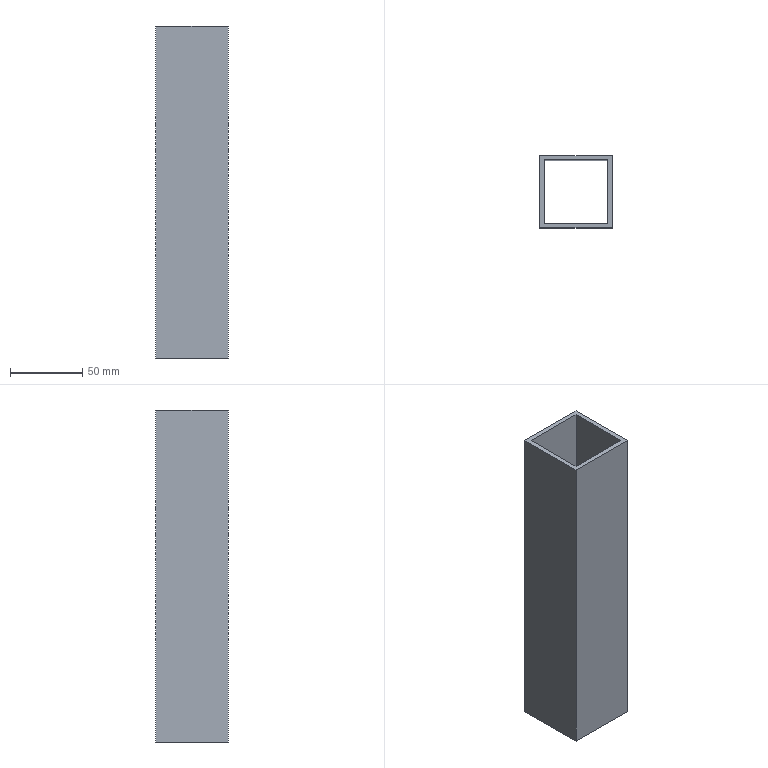Part | STEP file | BCC3 H19_1 | 1 solid | 10 faces | box 50 x 50 x 230 mm | volume 129720 mm3 | plane 10
STEP:
#1=CARTESIAN_POINT('',(0.,0.,0.));
#2=DIRECTION('',(0.,0.,1.));
#3=DIRECTION('',(1.,0.,0.));
#4=AXIS2_PLACEMENT_3D('',#1,#2,#3);
#5=CARTESIAN_POINT('',(-25.,25.,115.));
#6=VERTEX_POINT('',#5);
#7=CARTESIAN_POINT('',(-25.,-25.,115.));
#8=VERTEX_POINT('',#7);
#9=CARTESIAN_POINT('',(-25.,25.,115.));
#10=DIRECTION('',(0.,-1.,0.));
#11=VECTOR('',#10,1.);
#12=LINE('',#9,#11);
#13=CARTESIAN_POINT('',(0.,0.,115.));
#14=DIRECTION('',(0.,0.,1.));
#15=DIRECTION('',(1.,0.,0.));
#16=AXIS2_PLACEMENT_3D('',#13,#14,#15);
#17=PLANE('',#16);
#18=CARTESIAN_POINT('',(-25.,25.));
#19=DIRECTION('',(0.,-1.));
#20=VECTOR('',#19,1.);
#21=LINE('',#18,#20);
#22=(GEOMETRIC_REPRESENTATION_CONTEXT(2)PARAMETRIC_REPRESENTATION_CONTEXT()REPRESENTATION_CONTEXT('',''));
#23=DEFINITIONAL_REPRESENTATION('',(#21),#22);
#24=PCURVE('',#17,#23);
#25=CARTESIAN_POINT('',(-25.,25.,115.));
#26=DIRECTION('',(1.,0.,0.));
#27=DIRECTION('',(0.,1.,0.));
#28=AXIS2_PLACEMENT_3D('',#25,#26,#27);
#29=PLANE('',#28);
#30=CARTESIAN_POINT('',(0.,0.));
#31=DIRECTION('',(-1.,0.));
#32=VECTOR('',#31,1.);
#33=LINE('',#30,#32);
#34=(GEOMETRIC_REPRESENTATION_CONTEXT(2)PARAMETRIC_REPRESENTATION_CONTEXT()REPRESENTATION_CONTEXT('',''));
#35=DEFINITIONAL_REPRESENTATION('',(#33),#34);
#36=PCURVE('',#29,#35);
#37=SURFACE_CURVE('',#12,(#24,#36),.PCURVE_S1.);
#38=EDGE_CURVE('',#6,#8,#37,.T.);
#39=ORIENTED_EDGE('',*,*,#38,.T.);
#40=CARTESIAN_POINT('',(25.,-25.,115.));
#41=VERTEX_POINT('',#40);
#42=CARTESIAN_POINT('',(-25.,-25.,115.));
#43=DIRECTION('',(1.,0.,0.));
#44=VECTOR('',#43,1.);
#45=LINE('',#42,#44);
#46=CARTESIAN_POINT('',(-25.,-25.));
#47=DIRECTION('',(1.,0.));
#48=VECTOR('',#47,1.);
#49=LINE('',#46,#48);
#50=(GEOMETRIC_REPRESENTATION_CONTEXT(2)PARAMETRIC_REPRESENTATION_CONTEXT()REPRESENTATION_CONTEXT('',''));
#51=DEFINITIONAL_REPRESENTATION('',(#49),#50);
#52=PCURVE('',#17,#51);
#53=CARTESIAN_POINT('',(-25.,-25.,115.));
#54=DIRECTION('',(0.,1.,0.));
#55=DIRECTION('',(0.,0.,1.));
#56=AXIS2_PLACEMENT_3D('',#53,#54,#55);
#57=PLANE('',#56);
#58=CARTESIAN_POINT('',(0.,0.));
#59=DIRECTION('',(0.,1.));
#60=VECTOR('',#59,1.);
#61=LINE('',#58,#60);
#62=(GEOMETRIC_REPRESENTATION_CONTEXT(2)PARAMETRIC_REPRESENTATION_CONTEXT()REPRESENTATION_CONTEXT('',''));
#63=DEFINITIONAL_REPRESENTATION('',(#61),#62);
#64=PCURVE('',#57,#63);
#65=SURFACE_CURVE('',#45,(#52,#64),.PCURVE_S1.);
#66=EDGE_CURVE('',#8,#41,#65,.T.);
#67=ORIENTED_EDGE('',*,*,#66,.T.);
#68=CARTESIAN_POINT('',(25.,25.,115.));
#69=VERTEX_POINT('',#68);
#70=CARTESIAN_POINT('',(25.,25.,115.));
#71=DIRECTION('',(0.,1.,0.));
#72=VECTOR('',#71,1.);
#73=LINE('',#70,#72);
#74=CARTESIAN_POINT('',(25.,25.));
#75=DIRECTION('',(0.,1.));
#76=VECTOR('',#75,1.);
#77=LINE('',#74,#76);
#78=(GEOMETRIC_REPRESENTATION_CONTEXT(2)PARAMETRIC_REPRESENTATION_CONTEXT()REPRESENTATION_CONTEXT('',''));
#79=DEFINITIONAL_REPRESENTATION('',(#77),#78);
#80=PCURVE('',#17,#79);
#81=CARTESIAN_POINT('',(25.,25.,115.));
#82=DIRECTION('',(-1.,0.,0.));
#83=DIRECTION('',(0.,-1.,0.));
#84=AXIS2_PLACEMENT_3D('',#81,#82,#83);
#85=PLANE('',#84);
#86=CARTESIAN_POINT('',(0.,0.));
#87=DIRECTION('',(-1.,0.));
#88=VECTOR('',#87,1.);
#89=LINE('',#86,#88);
#90=(GEOMETRIC_REPRESENTATION_CONTEXT(2)PARAMETRIC_REPRESENTATION_CONTEXT()REPRESENTATION_CONTEXT('',''));
#91=DEFINITIONAL_REPRESENTATION('',(#89),#90);
#92=PCURVE('',#85,#91);
#93=SURFACE_CURVE('',#73,(#80,#92),.PCURVE_S1.);
#94=EDGE_CURVE('',#41,#69,#93,.T.);
#95=ORIENTED_EDGE('',*,*,#94,.T.);
#96=CARTESIAN_POINT('',(-25.,25.,115.));
#97=DIRECTION('',(-1.,0.,0.));
#98=VECTOR('',#97,1.);
#99=LINE('',#96,#98);
#100=CARTESIAN_POINT('',(-25.,25.));
#101=DIRECTION('',(-1.,0.));
#102=VECTOR('',#101,1.);
#103=LINE('',#100,#102);
#104=(GEOMETRIC_REPRESENTATION_CONTEXT(2)PARAMETRIC_REPRESENTATION_CONTEXT()REPRESENTATION_CONTEXT('',''));
#105=DEFINITIONAL_REPRESENTATION('',(#103),#104);
#106=PCURVE('',#17,#105);
#107=CARTESIAN_POINT('',(-25.,25.,115.));
#108=DIRECTION('',(0.,-1.,0.));
#109=DIRECTION('',(0.,0.,-1.));
#110=AXIS2_PLACEMENT_3D('',#107,#108,#109);
#111=PLANE('',#110);
#112=CARTESIAN_POINT('',(0.,0.));
#113=DIRECTION('',(0.,-1.));
#114=VECTOR('',#113,1.);
#115=LINE('',#112,#114);
#116=(GEOMETRIC_REPRESENTATION_CONTEXT(2)PARAMETRIC_REPRESENTATION_CONTEXT()REPRESENTATION_CONTEXT('',''));
#117=DEFINITIONAL_REPRESENTATION('',(#115),#116);
#118=PCURVE('',#111,#117);
#119=SURFACE_CURVE('',#99,(#106,#118),.PCURVE_S1.);
#120=EDGE_CURVE('',#69,#6,#119,.T.);
#121=ORIENTED_EDGE('',*,*,#120,.T.);
#122=EDGE_LOOP('',(#39,#67,#95,#121));
#123=FACE_BOUND('',#122,.T.);
#124=CARTESIAN_POINT('',(-22.,-22.,115.));
#125=VERTEX_POINT('',#124);
#126=CARTESIAN_POINT('',(22.,-22.,115.));
#127=VERTEX_POINT('',#126);
#128=CARTESIAN_POINT('',(-22.,-22.,115.));
#129=DIRECTION('',(1.,0.,0.));
#130=VECTOR('',#129,1.);
#131=LINE('',#128,#130);
#132=CARTESIAN_POINT('',(-22.,-22.));
#133=DIRECTION('',(1.,0.));
#134=VECTOR('',#133,1.);
#135=LINE('',#132,#134);
#136=(GEOMETRIC_REPRESENTATION_CONTEXT(2)PARAMETRIC_REPRESENTATION_CONTEXT()REPRESENTATION_CONTEXT('',''));
#137=DEFINITIONAL_REPRESENTATION('',(#135),#136);
#138=PCURVE('',#17,#137);
#139=CARTESIAN_POINT('',(-22.,-22.,115.));
#140=DIRECTION('',(0.,1.,0.));
#141=DIRECTION('',(-1.,0.,0.));
#142=AXIS2_PLACEMENT_3D('',#139,#140,#141);
#143=PLANE('',#142);
#144=CARTESIAN_POINT('',(0.,0.));
#145=DIRECTION('',(-1.,0.));
#146=VECTOR('',#145,1.);
#147=LINE('',#144,#146);
#148=(GEOMETRIC_REPRESENTATION_CONTEXT(2)PARAMETRIC_REPRESENTATION_CONTEXT()REPRESENTATION_CONTEXT('',''));
#149=DEFINITIONAL_REPRESENTATION('',(#147),#148);
#150=PCURVE('',#143,#149);
#151=SURFACE_CURVE('',#131,(#138,#150),.PCURVE_S1.);
#152=EDGE_CURVE('',#125,#127,#151,.T.);
#153=ORIENTED_EDGE('',*,*,#152,.F.);
#154=CARTESIAN_POINT('',(-22.,22.,115.));
#155=VERTEX_POINT('',#154);
#156=CARTESIAN_POINT('',(-22.,22.,115.));
#157=DIRECTION('',(0.,-1.,0.));
#158=VECTOR('',#157,1.);
#159=LINE('',#156,#158);
#160=CARTESIAN_POINT('',(-22.,22.));
#161=DIRECTION('',(0.,-1.));
#162=VECTOR('',#161,1.);
#163=LINE('',#160,#162);
#164=(GEOMETRIC_REPRESENTATION_CONTEXT(2)PARAMETRIC_REPRESENTATION_CONTEXT()REPRESENTATION_CONTEXT('',''));
#165=DEFINITIONAL_REPRESENTATION('',(#163),#164);
#166=PCURVE('',#17,#165);
#167=CARTESIAN_POINT('',(-22.,22.,115.));
#168=DIRECTION('',(1.,0.,0.));
#169=DIRECTION('',(0.,1.,0.));
#170=AXIS2_PLACEMENT_3D('',#167,#168,#169);
#171=PLANE('',#170);
#172=CARTESIAN_POINT('',(0.,0.));
#173=DIRECTION('',(-1.,0.));
#174=VECTOR('',#173,1.);
#175=LINE('',#172,#174);
#176=(GEOMETRIC_REPRESENTATION_CONTEXT(2)PARAMETRIC_REPRESENTATION_CONTEXT()REPRESENTATION_CONTEXT('',''));
#177=DEFINITIONAL_REPRESENTATION('',(#175),#176);
#178=PCURVE('',#171,#177);
#179=SURFACE_CURVE('',#159,(#166,#178),.PCURVE_S1.);
#180=EDGE_CURVE('',#155,#125,#179,.T.);
#181=ORIENTED_EDGE('',*,*,#180,.F.);
#182=CARTESIAN_POINT('',(22.,22.,115.));
#183=VERTEX_POINT('',#182);
#184=CARTESIAN_POINT('',(-22.,22.,115.));
#185=DIRECTION('',(-1.,0.,0.));
#186=VECTOR('',#185,1.);
#187=LINE('',#184,#186);
#188=CARTESIAN_POINT('',(-22.,22.));
#189=DIRECTION('',(-1.,0.));
#190=VECTOR('',#189,1.);
#191=LINE('',#188,#190);
#192=(GEOMETRIC_REPRESENTATION_CONTEXT(2)PARAMETRIC_REPRESENTATION_CONTEXT()REPRESENTATION_CONTEXT('',''));
#193=DEFINITIONAL_REPRESENTATION('',(#191),#192);
#194=PCURVE('',#17,#193);
#195=CARTESIAN_POINT('',(-22.,22.,115.));
#196=DIRECTION('',(0.,-1.,0.));
#197=DIRECTION('',(0.,0.,-1.));
#198=AXIS2_PLACEMENT_3D('',#195,#196,#197);
#199=PLANE('',#198);
#200=CARTESIAN_POINT('',(0.,0.));
#201=DIRECTION('',(0.,-1.));
#202=VECTOR('',#201,1.);
#203=LINE('',#200,#202);
#204=(GEOMETRIC_REPRESENTATION_CONTEXT(2)PARAMETRIC_REPRESENTATION_CONTEXT()REPRESENTATION_CONTEXT('',''));
#205=DEFINITIONAL_REPRESENTATION('',(#203),#204);
#206=PCURVE('',#199,#205);
#207=SURFACE_CURVE('',#187,(#194,#206),.PCURVE_S1.);
#208=EDGE_CURVE('',#183,#155,#207,.T.);
#209=ORIENTED_EDGE('',*,*,#208,.F.);
#210=CARTESIAN_POINT('',(22.,22.,115.));
#211=DIRECTION('',(0.,1.,0.));
#212=VECTOR('',#211,1.);
#213=LINE('',#210,#212);
#214=CARTESIAN_POINT('',(22.,22.));
#215=DIRECTION('',(0.,1.));
#216=VECTOR('',#215,1.);
#217=LINE('',#214,#216);
#218=(GEOMETRIC_REPRESENTATION_CONTEXT(2)PARAMETRIC_REPRESENTATION_CONTEXT()REPRESENTATION_CONTEXT('',''));
#219=DEFINITIONAL_REPRESENTATION('',(#217),#218);
#220=PCURVE('',#17,#219);
#221=CARTESIAN_POINT('',(22.,22.,115.));
#222=DIRECTION('',(-1.,0.,0.));
#223=DIRECTION('',(0.,-1.,0.));
#224=AXIS2_PLACEMENT_3D('',#221,#222,#223);
#225=PLANE('',#224);
#226=CARTESIAN_POINT('',(0.,0.));
#227=DIRECTION('',(-1.,0.));
#228=VECTOR('',#227,1.);
#229=LINE('',#226,#228);
#230=(GEOMETRIC_REPRESENTATION_CONTEXT(2)PARAMETRIC_REPRESENTATION_CONTEXT()REPRESENTATION_CONTEXT('',''));
#231=DEFINITIONAL_REPRESENTATION('',(#229),#230);
#232=PCURVE('',#225,#231);
#233=SURFACE_CURVE('',#213,(#220,#232),.PCURVE_S1.);
#234=EDGE_CURVE('',#127,#183,#233,.T.);
#235=ORIENTED_EDGE('',*,*,#234,.F.);
#236=EDGE_LOOP('',(#153,#181,#209,#235));
#237=FACE_BOUND('',#236,.T.);
#238=ADVANCED_FACE('',(#123,#237),#17,.T.);
#239=CARTESIAN_POINT('',(-25.,25.,-115.));
#240=VERTEX_POINT('',#239);
#241=CARTESIAN_POINT('',(-25.,-25.,-115.));
#242=VERTEX_POINT('',#241);
#243=CARTESIAN_POINT('',(-25.,25.,-115.));
#244=DIRECTION('',(0.,-1.,0.));
#245=VECTOR('',#244,1.);
#246=LINE('',#243,#245);
#247=CARTESIAN_POINT('',(0.,0.,-115.));
#248=DIRECTION('',(0.,0.,1.));
#249=DIRECTION('',(1.,0.,0.));
#250=AXIS2_PLACEMENT_3D('',#247,#248,#249);
#251=PLANE('',#250);
#252=CARTESIAN_POINT('',(-25.,25.));
#253=DIRECTION('',(0.,-1.));
#254=VECTOR('',#253,1.);
#255=LINE('',#252,#254);
#256=(GEOMETRIC_REPRESENTATION_CONTEXT(2)PARAMETRIC_REPRESENTATION_CONTEXT()REPRESENTATION_CONTEXT('',''));
#257=DEFINITIONAL_REPRESENTATION('',(#255),#256);
#258=PCURVE('',#251,#257);
#259=CARTESIAN_POINT('',(0.,-230.));
#260=DIRECTION('',(-1.,0.));
#261=VECTOR('',#260,1.);
#262=LINE('',#259,#261);
#263=(GEOMETRIC_REPRESENTATION_CONTEXT(2)PARAMETRIC_REPRESENTATION_CONTEXT()REPRESENTATION_CONTEXT('',''));
#264=DEFINITIONAL_REPRESENTATION('',(#262),#263);
#265=PCURVE('',#29,#264);
#266=SURFACE_CURVE('',#246,(#258,#265),.PCURVE_S1.);
#267=EDGE_CURVE('',#240,#242,#266,.T.);
#268=ORIENTED_EDGE('',*,*,#267,.F.);
#269=CARTESIAN_POINT('',(25.,25.,-115.));
#270=VERTEX_POINT('',#269);
#271=CARTESIAN_POINT('',(-25.,25.,-115.));
#272=DIRECTION('',(-1.,0.,0.));
#273=VECTOR('',#272,1.);
#274=LINE('',#271,#273);
#275=CARTESIAN_POINT('',(-25.,25.));
#276=DIRECTION('',(-1.,0.));
#277=VECTOR('',#276,1.);
#278=LINE('',#275,#277);
#279=(GEOMETRIC_REPRESENTATION_CONTEXT(2)PARAMETRIC_REPRESENTATION_CONTEXT()REPRESENTATION_CONTEXT('',''));
#280=DEFINITIONAL_REPRESENTATION('',(#278),#279);
#281=PCURVE('',#251,#280);
#282=CARTESIAN_POINT('',(230.,0.));
#283=DIRECTION('',(0.,-1.));
#284=VECTOR('',#283,1.);
#285=LINE('',#282,#284);
#286=(GEOMETRIC_REPRESENTATION_CONTEXT(2)PARAMETRIC_REPRESENTATION_CONTEXT()REPRESENTATION_CONTEXT('',''));
#287=DEFINITIONAL_REPRESENTATION('',(#285),#286);
#288=PCURVE('',#111,#287);
#289=SURFACE_CURVE('',#274,(#281,#288),.PCURVE_S1.);
#290=EDGE_CURVE('',#270,#240,#289,.T.);
#291=ORIENTED_EDGE('',*,*,#290,.F.);
#292=CARTESIAN_POINT('',(25.,-25.,-115.));
#293=VERTEX_POINT('',#292);
#294=CARTESIAN_POINT('',(25.,25.,-115.));
#295=DIRECTION('',(0.,1.,0.));
#296=VECTOR('',#295,1.);
#297=LINE('',#294,#296);
#298=CARTESIAN_POINT('',(25.,25.));
#299=DIRECTION('',(0.,1.));
#300=VECTOR('',#299,1.);
#301=LINE('',#298,#300);
#302=(GEOMETRIC_REPRESENTATION_CONTEXT(2)PARAMETRIC_REPRESENTATION_CONTEXT()REPRESENTATION_CONTEXT('',''));
#303=DEFINITIONAL_REPRESENTATION('',(#301),#302);
#304=PCURVE('',#251,#303);
#305=CARTESIAN_POINT('',(0.,-230.));
#306=DIRECTION('',(-1.,0.));
#307=VECTOR('',#306,1.);
#308=LINE('',#305,#307);
#309=(GEOMETRIC_REPRESENTATION_CONTEXT(2)PARAMETRIC_REPRESENTATION_CONTEXT()REPRESENTATION_CONTEXT('',''));
#310=DEFINITIONAL_REPRESENTATION('',(#308),#309);
#311=PCURVE('',#85,#310);
#312=SURFACE_CURVE('',#297,(#304,#311),.PCURVE_S1.);
#313=EDGE_CURVE('',#293,#270,#312,.T.);
#314=ORIENTED_EDGE('',*,*,#313,.F.);
#315=CARTESIAN_POINT('',(-25.,-25.,-115.));
#316=DIRECTION('',(1.,0.,0.));
#317=VECTOR('',#316,1.);
#318=LINE('',#315,#317);
#319=CARTESIAN_POINT('',(-25.,-25.));
#320=DIRECTION('',(1.,0.));
#321=VECTOR('',#320,1.);
#322=LINE('',#319,#321);
#323=(GEOMETRIC_REPRESENTATION_CONTEXT(2)PARAMETRIC_REPRESENTATION_CONTEXT()REPRESENTATION_CONTEXT('',''));
#324=DEFINITIONAL_REPRESENTATION('',(#322),#323);
#325=PCURVE('',#251,#324);
#326=CARTESIAN_POINT('',(-230.,0.));
#327=DIRECTION('',(0.,1.));
#328=VECTOR('',#327,1.);
#329=LINE('',#326,#328);
#330=(GEOMETRIC_REPRESENTATION_CONTEXT(2)PARAMETRIC_REPRESENTATION_CONTEXT()REPRESENTATION_CONTEXT('',''));
#331=DEFINITIONAL_REPRESENTATION('',(#329),#330);
#332=PCURVE('',#57,#331);
#333=SURFACE_CURVE('',#318,(#325,#332),.PCURVE_S1.);
#334=EDGE_CURVE('',#242,#293,#333,.T.);
#335=ORIENTED_EDGE('',*,*,#334,.F.);
#336=EDGE_LOOP('',(#268,#291,#314,#335));
#337=FACE_BOUND('',#336,.T.);
#338=CARTESIAN_POINT('',(-22.,22.,-115.));
#339=VERTEX_POINT('',#338);
#340=CARTESIAN_POINT('',(-22.,-22.,-115.));
#341=VERTEX_POINT('',#340);
#342=CARTESIAN_POINT('',(-22.,22.,-115.));
#343=DIRECTION('',(0.,-1.,0.));
#344=VECTOR('',#343,1.);
#345=LINE('',#342,#344);
#346=CARTESIAN_POINT('',(-22.,22.));
#347=DIRECTION('',(0.,-1.));
#348=VECTOR('',#347,1.);
#349=LINE('',#346,#348);
#350=(GEOMETRIC_REPRESENTATION_CONTEXT(2)PARAMETRIC_REPRESENTATION_CONTEXT()REPRESENTATION_CONTEXT('',''));
#351=DEFINITIONAL_REPRESENTATION('',(#349),#350);
#352=PCURVE('',#251,#351);
#353=CARTESIAN_POINT('',(0.,-230.));
#354=DIRECTION('',(-1.,0.));
#355=VECTOR('',#354,1.);
#356=LINE('',#353,#355);
#357=(GEOMETRIC_REPRESENTATION_CONTEXT(2)PARAMETRIC_REPRESENTATION_CONTEXT()REPRESENTATION_CONTEXT('',''));
#358=DEFINITIONAL_REPRESENTATION('',(#356),#357);
#359=PCURVE('',#171,#358);
#360=SURFACE_CURVE('',#345,(#352,#359),.PCURVE_S1.);
#361=EDGE_CURVE('',#339,#341,#360,.T.);
#362=ORIENTED_EDGE('',*,*,#361,.T.);
#363=CARTESIAN_POINT('',(22.,-22.,-115.));
#364=VERTEX_POINT('',#363);
#365=CARTESIAN_POINT('',(-22.,-22.,-115.));
#366=DIRECTION('',(1.,0.,0.));
#367=VECTOR('',#366,1.);
#368=LINE('',#365,#367);
#369=CARTESIAN_POINT('',(-22.,-22.));
#370=DIRECTION('',(1.,0.));
#371=VECTOR('',#370,1.);
#372=LINE('',#369,#371);
#373=(GEOMETRIC_REPRESENTATION_CONTEXT(2)PARAMETRIC_REPRESENTATION_CONTEXT()REPRESENTATION_CONTEXT('',''));
#374=DEFINITIONAL_REPRESENTATION('',(#372),#373);
#375=PCURVE('',#251,#374);
#376=CARTESIAN_POINT('',(0.,-230.));
#377=DIRECTION('',(-1.,0.));
#378=VECTOR('',#377,1.);
#379=LINE('',#376,#378);
#380=(GEOMETRIC_REPRESENTATION_CONTEXT(2)PARAMETRIC_REPRESENTATION_CONTEXT()REPRESENTATION_CONTEXT('',''));
#381=DEFINITIONAL_REPRESENTATION('',(#379),#380);
#382=PCURVE('',#143,#381);
#383=SURFACE_CURVE('',#368,(#375,#382),.PCURVE_S1.);
#384=EDGE_CURVE('',#341,#364,#383,.T.);
#385=ORIENTED_EDGE('',*,*,#384,.T.);
#386=CARTESIAN_POINT('',(22.,22.,-115.));
#387=VERTEX_POINT('',#386);
#388=CARTESIAN_POINT('',(22.,22.,-115.));
#389=DIRECTION('',(0.,1.,0.));
#390=VECTOR('',#389,1.);
#391=LINE('',#388,#390);
#392=CARTESIAN_POINT('',(22.,22.));
#393=DIRECTION('',(0.,1.));
#394=VECTOR('',#393,1.);
#395=LINE('',#392,#394);
#396=(GEOMETRIC_REPRESENTATION_CONTEXT(2)PARAMETRIC_REPRESENTATION_CONTEXT()REPRESENTATION_CONTEXT('',''));
#397=DEFINITIONAL_REPRESENTATION('',(#395),#396);
#398=PCURVE('',#251,#397);
#399=CARTESIAN_POINT('',(0.,-230.));
#400=DIRECTION('',(-1.,0.));
#401=VECTOR('',#400,1.);
#402=LINE('',#399,#401);
#403=(GEOMETRIC_REPRESENTATION_CONTEXT(2)PARAMETRIC_REPRESENTATION_CONTEXT()REPRESENTATION_CONTEXT('',''));
#404=DEFINITIONAL_REPRESENTATION('',(#402),#403);
#405=PCURVE('',#225,#404);
#406=SURFACE_CURVE('',#391,(#398,#405),.PCURVE_S1.);
#407=EDGE_CURVE('',#364,#387,#406,.T.);
#408=ORIENTED_EDGE('',*,*,#407,.T.);
#409=CARTESIAN_POINT('',(-22.,22.,-115.));
#410=DIRECTION('',(-1.,0.,0.));
#411=VECTOR('',#410,1.);
#412=LINE('',#409,#411);
#413=CARTESIAN_POINT('',(-22.,22.));
#414=DIRECTION('',(-1.,0.));
#415=VECTOR('',#414,1.);
#416=LINE('',#413,#415);
#417=(GEOMETRIC_REPRESENTATION_CONTEXT(2)PARAMETRIC_REPRESENTATION_CONTEXT()REPRESENTATION_CONTEXT('',''));
#418=DEFINITIONAL_REPRESENTATION('',(#416),#417);
#419=PCURVE('',#251,#418);
#420=CARTESIAN_POINT('',(230.,0.));
#421=DIRECTION('',(0.,-1.));
#422=VECTOR('',#421,1.);
#423=LINE('',#420,#422);
#424=(GEOMETRIC_REPRESENTATION_CONTEXT(2)PARAMETRIC_REPRESENTATION_CONTEXT()REPRESENTATION_CONTEXT('',''));
#425=DEFINITIONAL_REPRESENTATION('',(#423),#424);
#426=PCURVE('',#199,#425);
#427=SURFACE_CURVE('',#412,(#419,#426),.PCURVE_S1.);
#428=EDGE_CURVE('',#387,#339,#427,.T.);
#429=ORIENTED_EDGE('',*,*,#428,.T.);
#430=EDGE_LOOP('',(#362,#385,#408,#429));
#431=FACE_BOUND('',#430,.T.);
#432=ADVANCED_FACE('',(#337,#431),#251,.F.);
#433=ORIENTED_EDGE('',*,*,#267,.T.);
#434=CARTESIAN_POINT('',(-25.,-25.,115.));
#435=DIRECTION('',(0.,0.,-1.));
#436=VECTOR('',#435,1.);
#437=LINE('',#434,#436);
#438=CARTESIAN_POINT('',(-50.,0.));
#439=DIRECTION('',(0.,-1.));
#440=VECTOR('',#439,1.);
#441=LINE('',#438,#440);
#442=(GEOMETRIC_REPRESENTATION_CONTEXT(2)PARAMETRIC_REPRESENTATION_CONTEXT()REPRESENTATION_CONTEXT('',''));
#443=DEFINITIONAL_REPRESENTATION('',(#441),#442);
#444=PCURVE('',#29,#443);
#445=CARTESIAN_POINT('',(0.,0.));
#446=DIRECTION('',(-1.,0.));
#447=VECTOR('',#446,1.);
#448=LINE('',#445,#447);
#449=(GEOMETRIC_REPRESENTATION_CONTEXT(2)PARAMETRIC_REPRESENTATION_CONTEXT()REPRESENTATION_CONTEXT('',''));
#450=DEFINITIONAL_REPRESENTATION('',(#448),#449);
#451=PCURVE('',#57,#450);
#452=SURFACE_CURVE('',#437,(#444,#451),.PCURVE_S1.);
#453=EDGE_CURVE('',#8,#242,#452,.T.);
#454=ORIENTED_EDGE('',*,*,#453,.F.);
#455=ORIENTED_EDGE('',*,*,#38,.F.);
#456=CARTESIAN_POINT('',(-25.,25.,115.));
#457=DIRECTION('',(0.,0.,-1.));
#458=VECTOR('',#457,1.);
#459=LINE('',#456,#458);
#460=CARTESIAN_POINT('',(0.,0.));
#461=DIRECTION('',(0.,-1.));
#462=VECTOR('',#461,1.);
#463=LINE('',#460,#462);
#464=(GEOMETRIC_REPRESENTATION_CONTEXT(2)PARAMETRIC_REPRESENTATION_CONTEXT()REPRESENTATION_CONTEXT('',''));
#465=DEFINITIONAL_REPRESENTATION('',(#463),#464);
#466=PCURVE('',#29,#465);
#467=CARTESIAN_POINT('',(0.,0.));
#468=DIRECTION('',(1.,0.));
#469=VECTOR('',#468,1.);
#470=LINE('',#467,#469);
#471=(GEOMETRIC_REPRESENTATION_CONTEXT(2)PARAMETRIC_REPRESENTATION_CONTEXT()REPRESENTATION_CONTEXT('',''));
#472=DEFINITIONAL_REPRESENTATION('',(#470),#471);
#473=PCURVE('',#111,#472);
#474=SURFACE_CURVE('',#459,(#466,#473),.PCURVE_S1.);
#475=EDGE_CURVE('',#6,#240,#474,.T.);
#476=ORIENTED_EDGE('',*,*,#475,.T.);
#477=EDGE_LOOP('',(#433,#454,#455,#476));
#478=FACE_BOUND('',#477,.T.);
#479=ADVANCED_FACE('',(#478),#29,.F.);
#480=ORIENTED_EDGE('',*,*,#334,.T.);
#481=CARTESIAN_POINT('',(25.,-25.,115.));
#482=DIRECTION('',(0.,0.,-1.));
#483=VECTOR('',#482,1.);
#484=LINE('',#481,#483);
#485=CARTESIAN_POINT('',(0.,50.));
#486=DIRECTION('',(-1.,0.));
#487=VECTOR('',#486,1.);
#488=LINE('',#485,#487);
#489=(GEOMETRIC_REPRESENTATION_CONTEXT(2)PARAMETRIC_REPRESENTATION_CONTEXT()REPRESENTATION_CONTEXT('',''));
#490=DEFINITIONAL_REPRESENTATION('',(#488),#489);
#491=PCURVE('',#57,#490);
#492=CARTESIAN_POINT('',(50.,0.));
#493=DIRECTION('',(0.,-1.));
#494=VECTOR('',#493,1.);
#495=LINE('',#492,#494);
#496=(GEOMETRIC_REPRESENTATION_CONTEXT(2)PARAMETRIC_REPRESENTATION_CONTEXT()REPRESENTATION_CONTEXT('',''));
#497=DEFINITIONAL_REPRESENTATION('',(#495),#496);
#498=PCURVE('',#85,#497);
#499=SURFACE_CURVE('',#484,(#491,#498),.PCURVE_S1.);
#500=EDGE_CURVE('',#41,#293,#499,.T.);
#501=ORIENTED_EDGE('',*,*,#500,.F.);
#502=ORIENTED_EDGE('',*,*,#66,.F.);
#503=ORIENTED_EDGE('',*,*,#453,.T.);
#504=EDGE_LOOP('',(#480,#501,#502,#503));
#505=FACE_BOUND('',#504,.T.);
#506=ADVANCED_FACE('',(#505),#57,.F.);
#507=ORIENTED_EDGE('',*,*,#313,.T.);
#508=CARTESIAN_POINT('',(25.,25.,115.));
#509=DIRECTION('',(0.,0.,-1.));
#510=VECTOR('',#509,1.);
#511=LINE('',#508,#510);
#512=CARTESIAN_POINT('',(0.,0.));
#513=DIRECTION('',(0.,-1.));
#514=VECTOR('',#513,1.);
#515=LINE('',#512,#514);
#516=(GEOMETRIC_REPRESENTATION_CONTEXT(2)PARAMETRIC_REPRESENTATION_CONTEXT()REPRESENTATION_CONTEXT('',''));
#517=DEFINITIONAL_REPRESENTATION('',(#515),#516);
#518=PCURVE('',#85,#517);
#519=CARTESIAN_POINT('',(0.,50.));
#520=DIRECTION('',(1.,0.));
#521=VECTOR('',#520,1.);
#522=LINE('',#519,#521);
#523=(GEOMETRIC_REPRESENTATION_CONTEXT(2)PARAMETRIC_REPRESENTATION_CONTEXT()REPRESENTATION_CONTEXT('',''));
#524=DEFINITIONAL_REPRESENTATION('',(#522),#523);
#525=PCURVE('',#111,#524);
#526=SURFACE_CURVE('',#511,(#518,#525),.PCURVE_S1.);
#527=EDGE_CURVE('',#69,#270,#526,.T.);
#528=ORIENTED_EDGE('',*,*,#527,.F.);
#529=ORIENTED_EDGE('',*,*,#94,.F.);
#530=ORIENTED_EDGE('',*,*,#500,.T.);
#531=EDGE_LOOP('',(#507,#528,#529,#530));
#532=FACE_BOUND('',#531,.T.);
#533=ADVANCED_FACE('',(#532),#85,.F.);
#534=ORIENTED_EDGE('',*,*,#290,.T.);
#535=ORIENTED_EDGE('',*,*,#475,.F.);
#536=ORIENTED_EDGE('',*,*,#120,.F.);
#537=ORIENTED_EDGE('',*,*,#527,.T.);
#538=EDGE_LOOP('',(#534,#535,#536,#537));
#539=FACE_BOUND('',#538,.T.);
#540=ADVANCED_FACE('',(#539),#111,.F.);
#541=ORIENTED_EDGE('',*,*,#361,.F.);
#542=CARTESIAN_POINT('',(-22.,22.,115.));
#543=DIRECTION('',(0.,0.,-1.));
#544=VECTOR('',#543,1.);
#545=LINE('',#542,#544);
#546=CARTESIAN_POINT('',(0.,0.));
#547=DIRECTION('',(0.,-1.));
#548=VECTOR('',#547,1.);
#549=LINE('',#546,#548);
#550=(GEOMETRIC_REPRESENTATION_CONTEXT(2)PARAMETRIC_REPRESENTATION_CONTEXT()REPRESENTATION_CONTEXT('',''));
#551=DEFINITIONAL_REPRESENTATION('',(#549),#550);
#552=PCURVE('',#171,#551);
#553=CARTESIAN_POINT('',(0.,0.));
#554=DIRECTION('',(1.,0.));
#555=VECTOR('',#554,1.);
#556=LINE('',#553,#555);
#557=(GEOMETRIC_REPRESENTATION_CONTEXT(2)PARAMETRIC_REPRESENTATION_CONTEXT()REPRESENTATION_CONTEXT('',''));
#558=DEFINITIONAL_REPRESENTATION('',(#556),#557);
#559=PCURVE('',#199,#558);
#560=SURFACE_CURVE('',#545,(#552,#559),.PCURVE_S1.);
#561=EDGE_CURVE('',#155,#339,#560,.T.);
#562=ORIENTED_EDGE('',*,*,#561,.F.);
#563=ORIENTED_EDGE('',*,*,#180,.T.);
#564=CARTESIAN_POINT('',(-22.,-22.,115.));
#565=DIRECTION('',(0.,0.,-1.));
#566=VECTOR('',#565,1.);
#567=LINE('',#564,#566);
#568=CARTESIAN_POINT('',(-44.,0.));
#569=DIRECTION('',(0.,-1.));
#570=VECTOR('',#569,1.);
#571=LINE('',#568,#570);
#572=(GEOMETRIC_REPRESENTATION_CONTEXT(2)PARAMETRIC_REPRESENTATION_CONTEXT()REPRESENTATION_CONTEXT('',''));
#573=DEFINITIONAL_REPRESENTATION('',(#571),#572);
#574=PCURVE('',#171,#573);
#575=CARTESIAN_POINT('',(0.,0.));
#576=DIRECTION('',(0.,-1.));
#577=VECTOR('',#576,1.);
#578=LINE('',#575,#577);
#579=(GEOMETRIC_REPRESENTATION_CONTEXT(2)PARAMETRIC_REPRESENTATION_CONTEXT()REPRESENTATION_CONTEXT('',''));
#580=DEFINITIONAL_REPRESENTATION('',(#578),#579);
#581=PCURVE('',#143,#580);
#582=SURFACE_CURVE('',#567,(#574,#581),.PCURVE_S1.);
#583=EDGE_CURVE('',#125,#341,#582,.T.);
#584=ORIENTED_EDGE('',*,*,#583,.T.);
#585=EDGE_LOOP('',(#541,#562,#563,#584));
#586=FACE_BOUND('',#585,.T.);
#587=ADVANCED_FACE('',(#586),#171,.T.);
#588=ORIENTED_EDGE('',*,*,#384,.F.);
#589=ORIENTED_EDGE('',*,*,#583,.F.);
#590=ORIENTED_EDGE('',*,*,#152,.T.);
#591=CARTESIAN_POINT('',(22.,-22.,115.));
#592=DIRECTION('',(0.,0.,-1.));
#593=VECTOR('',#592,1.);
#594=LINE('',#591,#593);
#595=CARTESIAN_POINT('',(-44.,0.));
#596=DIRECTION('',(0.,-1.));
#597=VECTOR('',#596,1.);
#598=LINE('',#595,#597);
#599=(GEOMETRIC_REPRESENTATION_CONTEXT(2)PARAMETRIC_REPRESENTATION_CONTEXT()REPRESENTATION_CONTEXT('',''));
#600=DEFINITIONAL_REPRESENTATION('',(#598),#599);
#601=PCURVE('',#143,#600);
#602=CARTESIAN_POINT('',(44.,0.));
#603=DIRECTION('',(0.,-1.));
#604=VECTOR('',#603,1.);
#605=LINE('',#602,#604);
#606=(GEOMETRIC_REPRESENTATION_CONTEXT(2)PARAMETRIC_REPRESENTATION_CONTEXT()REPRESENTATION_CONTEXT('',''));
#607=DEFINITIONAL_REPRESENTATION('',(#605),#606);
#608=PCURVE('',#225,#607);
#609=SURFACE_CURVE('',#594,(#601,#608),.PCURVE_S1.);
#610=EDGE_CURVE('',#127,#364,#609,.T.);
#611=ORIENTED_EDGE('',*,*,#610,.T.);
#612=EDGE_LOOP('',(#588,#589,#590,#611));
#613=FACE_BOUND('',#612,.T.);
#614=ADVANCED_FACE('',(#613),#143,.T.);
#615=ORIENTED_EDGE('',*,*,#407,.F.);
#616=ORIENTED_EDGE('',*,*,#610,.F.);
#617=ORIENTED_EDGE('',*,*,#234,.T.);
#618=CARTESIAN_POINT('',(22.,22.,115.));
#619=DIRECTION('',(0.,0.,-1.));
#620=VECTOR('',#619,1.);
#621=LINE('',#618,#620);
#622=CARTESIAN_POINT('',(0.,0.));
#623=DIRECTION('',(0.,-1.));
#624=VECTOR('',#623,1.);
#625=LINE('',#622,#624);
#626=(GEOMETRIC_REPRESENTATION_CONTEXT(2)PARAMETRIC_REPRESENTATION_CONTEXT()REPRESENTATION_CONTEXT('',''));
#627=DEFINITIONAL_REPRESENTATION('',(#625),#626);
#628=PCURVE('',#225,#627);
#629=CARTESIAN_POINT('',(0.,44.));
#630=DIRECTION('',(1.,0.));
#631=VECTOR('',#630,1.);
#632=LINE('',#629,#631);
#633=(GEOMETRIC_REPRESENTATION_CONTEXT(2)PARAMETRIC_REPRESENTATION_CONTEXT()REPRESENTATION_CONTEXT('',''));
#634=DEFINITIONAL_REPRESENTATION('',(#632),#633);
#635=PCURVE('',#199,#634);
#636=SURFACE_CURVE('',#621,(#628,#635),.PCURVE_S1.);
#637=EDGE_CURVE('',#183,#387,#636,.T.);
#638=ORIENTED_EDGE('',*,*,#637,.T.);
#639=EDGE_LOOP('',(#615,#616,#617,#638));
#640=FACE_BOUND('',#639,.T.);
#641=ADVANCED_FACE('',(#640),#225,.T.);
#642=ORIENTED_EDGE('',*,*,#428,.F.);
#643=ORIENTED_EDGE('',*,*,#637,.F.);
#644=ORIENTED_EDGE('',*,*,#208,.T.);
#645=ORIENTED_EDGE('',*,*,#561,.T.);
#646=EDGE_LOOP('',(#642,#643,#644,#645));
#647=FACE_BOUND('',#646,.T.);
#648=ADVANCED_FACE('',(#647),#199,.T.);
#649=CLOSED_SHELL('',(#238,#432,#479,#506,#533,#540,#587,#614,#641,#648));
#650=MANIFOLD_SOLID_BREP('',#649);
#651=(LENGTH_UNIT()NAMED_UNIT(*)SI_UNIT(.MILLI.,.METRE.));
#652=UNCERTAINTY_MEASURE_WITH_UNIT(LENGTH_MEASURE(0.0000001),#651,'','');
#653=(NAMED_UNIT(*)PLANE_ANGLE_UNIT()SI_UNIT($,.RADIAN.));
#654=(NAMED_UNIT(*)SI_UNIT($,.STERADIAN.)SOLID_ANGLE_UNIT());
#655=(GEOMETRIC_REPRESENTATION_CONTEXT(3)GLOBAL_UNCERTAINTY_ASSIGNED_CONTEXT((#652))GLOBAL_UNIT_ASSIGNED_CONTEXT((#651,#653,#654))REPRESENTATION_CONTEXT('',''));
#656=ADVANCED_BREP_SHAPE_REPRESENTATION('',(#4,#650),#655);